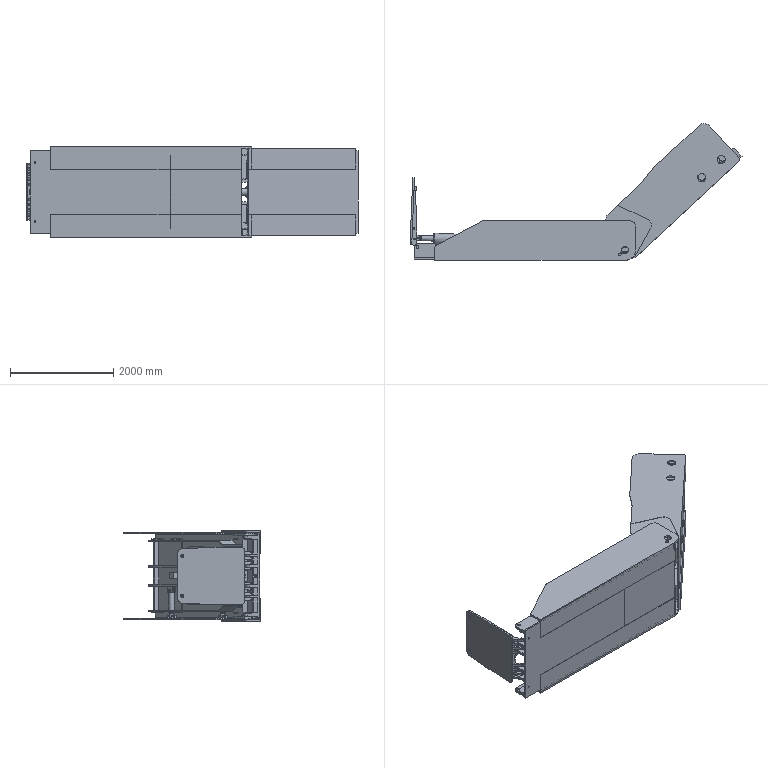Part | NX | features 掩护梁 16, 侧推千斤顶活塞 2, 侧推千斤顶活塞销 2, 侧推千斤顶缸 2, 侧推千斤顶缸销 2, 平衡千斤顶活塞 2, 平衡千斤顶活塞销 2, 平衡千斤顶缸 2, 平衡千斤顶缸销 2, 护帮千斤顶活塞 2, 护帮千斤顶缸 2, 护邦千斤顶活塞销 2, 护邦千斤顶滑块 2, 护邦千斤顶滑块销 2, 护邦销 2, 掩护梁侧护板右 2, 掩护梁侧护板左 2, 梁销挡板 2, 顶梁 2, 顶梁侧护板右 2, 顶梁侧护板左 2, 顶梁掩护板柱销 2 | 46 solids | 1508 faces | box 6418 x 2642 x 1741 mm | volume 733546494 mm3 | plane 1065 | cylinder 357 | cone 64 | sphere 10 | spline 9 | torus 3 | commonest cylinder face diameters 30 x35 20 x25 40 x21 107 x16 10 x12 145 x12